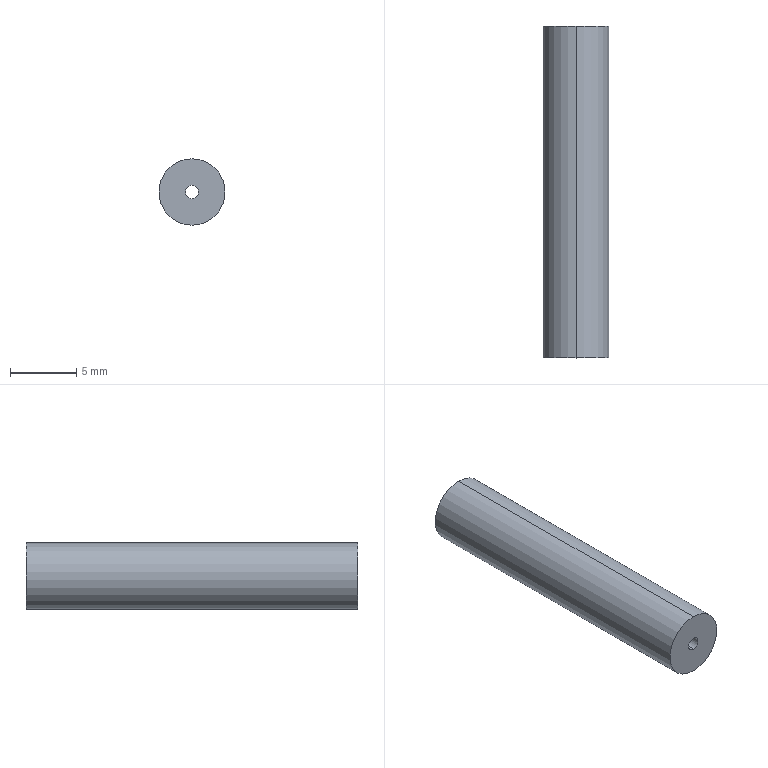Part | SolidWorks | features Extrusion 1, ICE 1 | 1 solid | 9 faces | box 5 x 25 x 5 mm | volume 326.726 mm3 | cylinder 6 | plane 3 | commonest cylinder face diameters 1 x2 3 x2 5 x2
STEP:
#1=CARTESIAN_POINT('',(0.,2.,0.5));
#2=VERTEX_POINT('',#1);
#3=CARTESIAN_POINT('',(0.,2.,-0.5));
#4=VERTEX_POINT('',#3);
#5=CARTESIAN_POINT('',(0.,2.,0.));
#6=DIRECTION('',(0.,-1.,0.));
#7=DIRECTION('',(0.,0.,-1.));
#8=AXIS2_PLACEMENT_3D('',#5,#6,#7);
#9=CIRCLE('',#8,0.5);
#10=EDGE_CURVE('',#2,#4,#9,.T.);
#11=ORIENTED_EDGE('',*,*,#10,.F.);
#12=CARTESIAN_POINT('',(0.,0.,0.5));
#13=VERTEX_POINT('',#12);
#14=CARTESIAN_POINT('',(0.,2.,0.5));
#15=DIRECTION('',(0.,-1.,0.));
#16=VECTOR('',#15,1000.);
#17=LINE('',#14,#16);
#18=EDGE_CURVE('',#2,#13,#17,.T.);
#19=ORIENTED_EDGE('',*,*,#18,.T.);
#20=CARTESIAN_POINT('',(0.,0.,-0.5));
#21=VERTEX_POINT('',#20);
#22=CARTESIAN_POINT('',(0.,0.,0.));
#23=DIRECTION('',(0.,-1.,0.));
#24=DIRECTION('',(0.,0.,-1.));
#25=AXIS2_PLACEMENT_3D('',#22,#23,#24);
#26=CIRCLE('',#25,0.5);
#27=EDGE_CURVE('',#13,#21,#26,.T.);
#28=ORIENTED_EDGE('',*,*,#27,.T.);
#29=CARTESIAN_POINT('',(0.,2.,-0.5));
#30=DIRECTION('',(0.,-1.,0.));
#31=VECTOR('',#30,1000.);
#32=LINE('',#29,#31);
#33=EDGE_CURVE('',#4,#21,#32,.T.);
#34=ORIENTED_EDGE('',*,*,#33,.F.);
#35=EDGE_LOOP('',(#11,#19,#28,#34));
#36=FACE_OUTER_BOUND('',#35,.T.);
#37=CARTESIAN_POINT('',(0.,2.,0.));
#38=DIRECTION('',(0.,-1.,0.));
#39=DIRECTION('',(0.,0.,-1.));
#40=AXIS2_PLACEMENT_3D('',#37,#38,#39);
#41=CYLINDRICAL_SURFACE('',#40,0.5);
#42=ADVANCED_FACE('',(#36),#41,.F.);
#43=CARTESIAN_POINT('',(0.,25.,2.5));
#44=VERTEX_POINT('',#43);
#45=CARTESIAN_POINT('',(0.,25.,-2.5));
#46=VERTEX_POINT('',#45);
#47=CARTESIAN_POINT('',(0.,25.,0.));
#48=DIRECTION('',(0.,1.,0.));
#49=DIRECTION('',(0.,0.,1.));
#50=AXIS2_PLACEMENT_3D('',#47,#48,#49);
#51=CIRCLE('',#50,2.5);
#52=EDGE_CURVE('',#44,#46,#51,.T.);
#53=ORIENTED_EDGE('',*,*,#52,.F.);
#54=CARTESIAN_POINT('',(0.,0.,2.5));
#55=VERTEX_POINT('',#54);
#56=CARTESIAN_POINT('',(0.,25.,2.5));
#57=DIRECTION('',(0.,-1.,0.));
#58=VECTOR('',#57,1000.);
#59=LINE('',#56,#58);
#60=EDGE_CURVE('',#44,#55,#59,.T.);
#61=ORIENTED_EDGE('',*,*,#60,.T.);
#62=CARTESIAN_POINT('',(0.,0.,-2.5));
#63=VERTEX_POINT('',#62);
#64=CARTESIAN_POINT('',(0.,0.,0.));
#65=DIRECTION('',(0.,1.,0.));
#66=DIRECTION('',(0.,0.,1.));
#67=AXIS2_PLACEMENT_3D('',#64,#65,#66);
#68=CIRCLE('',#67,2.5);
#69=EDGE_CURVE('',#55,#63,#68,.T.);
#70=ORIENTED_EDGE('',*,*,#69,.T.);
#71=CARTESIAN_POINT('',(0.,25.,-2.5));
#72=DIRECTION('',(0.,-1.,0.));
#73=VECTOR('',#72,1000.);
#74=LINE('',#71,#73);
#75=EDGE_CURVE('',#46,#63,#74,.T.);
#76=ORIENTED_EDGE('',*,*,#75,.F.);
#77=EDGE_LOOP('',(#53,#61,#70,#76));
#78=FACE_OUTER_BOUND('',#77,.T.);
#79=CARTESIAN_POINT('',(0.,25.,0.));
#80=DIRECTION('',(0.,-1.,0.));
#81=DIRECTION('',(0.,0.,-1.));
#82=AXIS2_PLACEMENT_3D('',#79,#80,#81);
#83=CYLINDRICAL_SURFACE('',#82,2.5);
#84=ADVANCED_FACE('',(#78),#83,.T.);
#85=CARTESIAN_POINT('',(0.,25.,-1.5));
#86=VERTEX_POINT('',#85);
#87=CARTESIAN_POINT('',(0.,25.,1.5));
#88=VERTEX_POINT('',#87);
#89=CARTESIAN_POINT('',(0.,25.,0.));
#90=DIRECTION('',(0.,1.,0.));
#91=DIRECTION('',(0.,0.,1.));
#92=AXIS2_PLACEMENT_3D('',#89,#90,#91);
#93=CIRCLE('',#92,1.5);
#94=EDGE_CURVE('',#86,#88,#93,.T.);
#95=ORIENTED_EDGE('',*,*,#94,.T.);
#96=CARTESIAN_POINT('',(0.,2.,1.5));
#97=VERTEX_POINT('',#96);
#98=CARTESIAN_POINT('',(0.,25.,1.5));
#99=DIRECTION('',(0.,-1.,0.));
#100=VECTOR('',#99,1000.);
#101=LINE('',#98,#100);
#102=EDGE_CURVE('',#88,#97,#101,.T.);
#103=ORIENTED_EDGE('',*,*,#102,.T.);
#104=CARTESIAN_POINT('',(0.,2.,-1.5));
#105=VERTEX_POINT('',#104);
#106=CARTESIAN_POINT('',(0.,2.,0.));
#107=DIRECTION('',(0.,-1.,0.));
#108=DIRECTION('',(0.,0.,-1.));
#109=AXIS2_PLACEMENT_3D('',#106,#107,#108);
#110=CIRCLE('',#109,1.5);
#111=EDGE_CURVE('',#97,#105,#110,.T.);
#112=ORIENTED_EDGE('',*,*,#111,.T.);
#113=CARTESIAN_POINT('',(0.,25.,-1.5));
#114=DIRECTION('',(0.,-1.,0.));
#115=VECTOR('',#114,1000.);
#116=LINE('',#113,#115);
#117=EDGE_CURVE('',#86,#105,#116,.T.);
#118=ORIENTED_EDGE('',*,*,#117,.F.);
#119=EDGE_LOOP('',(#95,#103,#112,#118));
#120=FACE_OUTER_BOUND('',#119,.T.);
#121=CARTESIAN_POINT('',(0.,25.,0.));
#122=DIRECTION('',(0.,-1.,0.));
#123=DIRECTION('',(0.,0.,-1.));
#124=AXIS2_PLACEMENT_3D('',#121,#122,#123);
#125=CYLINDRICAL_SURFACE('',#124,1.5);
#126=ADVANCED_FACE('',(#120),#125,.F.);
#127=ORIENTED_EDGE('',*,*,#102,.F.);
#128=CARTESIAN_POINT('',(0.,25.,0.));
#129=DIRECTION('',(0.,1.,0.));
#130=DIRECTION('',(0.,0.,1.));
#131=AXIS2_PLACEMENT_3D('',#128,#129,#130);
#132=CIRCLE('',#131,1.5);
#133=EDGE_CURVE('',#88,#86,#132,.T.);
#134=ORIENTED_EDGE('',*,*,#133,.T.);
#135=ORIENTED_EDGE('',*,*,#117,.T.);
#136=CARTESIAN_POINT('',(0.,2.,0.));
#137=DIRECTION('',(0.,-1.,0.));
#138=DIRECTION('',(0.,0.,-1.));
#139=AXIS2_PLACEMENT_3D('',#136,#137,#138);
#140=CIRCLE('',#139,1.5);
#141=EDGE_CURVE('',#105,#97,#140,.T.);
#142=ORIENTED_EDGE('',*,*,#141,.T.);
#143=EDGE_LOOP('',(#127,#134,#135,#142));
#144=FACE_OUTER_BOUND('',#143,.T.);
#145=CARTESIAN_POINT('',(0.,25.,0.));
#146=DIRECTION('',(0.,-1.,0.));
#147=DIRECTION('',(0.,0.,-1.));
#148=AXIS2_PLACEMENT_3D('',#145,#146,#147);
#149=CYLINDRICAL_SURFACE('',#148,1.5);
#150=ADVANCED_FACE('',(#144),#149,.F.);
#151=CARTESIAN_POINT('',(0.,25.,0.));
#152=DIRECTION('',(0.,1.,0.));
#153=DIRECTION('',(0.,0.,1.));
#154=AXIS2_PLACEMENT_3D('',#151,#152,#153);
#155=CIRCLE('',#154,2.5);
#156=EDGE_CURVE('',#46,#44,#155,.T.);
#157=ORIENTED_EDGE('',*,*,#156,.T.);
#158=ORIENTED_EDGE('',*,*,#52,.T.);
#159=EDGE_LOOP('',(#157,#158));
#160=FACE_OUTER_BOUND('',#159,.T.);
#161=ORIENTED_EDGE('',*,*,#94,.F.);
#162=ORIENTED_EDGE('',*,*,#133,.F.);
#163=EDGE_LOOP('',(#161,#162));
#164=FACE_BOUND('',#163,.T.);
#165=CARTESIAN_POINT('',(0.,25.,0.));
#166=DIRECTION('',(0.,1.,0.));
#167=DIRECTION('',(0.,0.,1.));
#168=AXIS2_PLACEMENT_3D('',#165,#166,#167);
#169=PLANE('',#168);
#170=ADVANCED_FACE('',(#160,#164),#169,.T.);
#171=CARTESIAN_POINT('',(0.,0.,0.));
#172=DIRECTION('',(0.,1.,0.));
#173=DIRECTION('',(0.,0.,1.));
#174=AXIS2_PLACEMENT_3D('',#171,#172,#173);
#175=CIRCLE('',#174,2.5);
#176=EDGE_CURVE('',#63,#55,#175,.T.);
#177=ORIENTED_EDGE('',*,*,#176,.F.);
#178=ORIENTED_EDGE('',*,*,#69,.F.);
#179=EDGE_LOOP('',(#177,#178));
#180=FACE_OUTER_BOUND('',#179,.T.);
#181=CARTESIAN_POINT('',(0.,0.,0.));
#182=DIRECTION('',(0.,-1.,0.));
#183=DIRECTION('',(0.,0.,-1.));
#184=AXIS2_PLACEMENT_3D('',#181,#182,#183);
#185=CIRCLE('',#184,0.5);
#186=EDGE_CURVE('',#21,#13,#185,.T.);
#187=ORIENTED_EDGE('',*,*,#186,.F.);
#188=ORIENTED_EDGE('',*,*,#27,.F.);
#189=EDGE_LOOP('',(#187,#188));
#190=FACE_BOUND('',#189,.T.);
#191=CARTESIAN_POINT('',(0.,0.,0.));
#192=DIRECTION('',(0.,1.,0.));
#193=DIRECTION('',(0.,0.,1.));
#194=AXIS2_PLACEMENT_3D('',#191,#192,#193);
#195=PLANE('',#194);
#196=ADVANCED_FACE('',(#180,#190),#195,.F.);
#197=ORIENTED_EDGE('',*,*,#60,.F.);
#198=ORIENTED_EDGE('',*,*,#156,.F.);
#199=ORIENTED_EDGE('',*,*,#75,.T.);
#200=ORIENTED_EDGE('',*,*,#176,.T.);
#201=EDGE_LOOP('',(#197,#198,#199,#200));
#202=FACE_OUTER_BOUND('',#201,.T.);
#203=CARTESIAN_POINT('',(0.,25.,0.));
#204=DIRECTION('',(0.,-1.,0.));
#205=DIRECTION('',(0.,0.,-1.));
#206=AXIS2_PLACEMENT_3D('',#203,#204,#205);
#207=CYLINDRICAL_SURFACE('',#206,2.5);
#208=ADVANCED_FACE('',(#202),#207,.T.);
#209=CARTESIAN_POINT('',(0.,2.,0.));
#210=DIRECTION('',(0.,-1.,0.));
#211=DIRECTION('',(0.,0.,-1.));
#212=AXIS2_PLACEMENT_3D('',#209,#210,#211);
#213=CIRCLE('',#212,0.5);
#214=EDGE_CURVE('',#4,#2,#213,.T.);
#215=ORIENTED_EDGE('',*,*,#214,.T.);
#216=ORIENTED_EDGE('',*,*,#10,.T.);
#217=EDGE_LOOP('',(#215,#216));
#218=FACE_BOUND('',#217,.T.);
#219=ORIENTED_EDGE('',*,*,#141,.F.);
#220=ORIENTED_EDGE('',*,*,#111,.F.);
#221=EDGE_LOOP('',(#219,#220));
#222=FACE_OUTER_BOUND('',#221,.T.);
#223=CARTESIAN_POINT('',(0.,2.,0.));
#224=DIRECTION('',(0.,-1.,0.));
#225=DIRECTION('',(0.,0.,-1.));
#226=AXIS2_PLACEMENT_3D('',#223,#224,#225);
#227=PLANE('',#226);
#228=ADVANCED_FACE('',(#218,#222),#227,.F.);
#229=ORIENTED_EDGE('',*,*,#18,.F.);
#230=ORIENTED_EDGE('',*,*,#214,.F.);
#231=ORIENTED_EDGE('',*,*,#33,.T.);
#232=ORIENTED_EDGE('',*,*,#186,.T.);
#233=EDGE_LOOP('',(#229,#230,#231,#232));
#234=FACE_OUTER_BOUND('',#233,.T.);
#235=CARTESIAN_POINT('',(0.,2.,0.));
#236=DIRECTION('',(0.,-1.,0.));
#237=DIRECTION('',(0.,0.,-1.));
#238=AXIS2_PLACEMENT_3D('',#235,#236,#237);
#239=CYLINDRICAL_SURFACE('',#238,0.5);
#240=ADVANCED_FACE('',(#234),#239,.F.);
#241=CLOSED_SHELL('',(#42,#84,#126,#150,#170,#196,#208,#228,#240));
#242=MANIFOLD_SOLID_BREP('',#241);
#243=CARTESIAN_POINT('',(0.,0.,0.));
#244=DIRECTION('',(0.,0.,1.));
#245=DIRECTION('',(1.,0.,0.));
#246=AXIS2_PLACEMENT_3D('',#243,#244,#245);
#247=(LENGTH_UNIT()NAMED_UNIT(*)SI_UNIT(.MILLI.,.METRE.));
#248=UNCERTAINTY_MEASURE_WITH_UNIT(LENGTH_MEASURE(0.00001),#247,'','');
#249=(NAMED_UNIT(*)PLANE_ANGLE_UNIT()SI_UNIT($,.RADIAN.));
#250=(NAMED_UNIT(*)SI_UNIT($,.STERADIAN.)SOLID_ANGLE_UNIT());
#251=(GEOMETRIC_REPRESENTATION_CONTEXT(3)GLOBAL_UNCERTAINTY_ASSIGNED_CONTEXT((#248))GLOBAL_UNIT_ASSIGNED_CONTEXT((#247,#249,#250))REPRESENTATION_CONTEXT('',''));
#252=ADVANCED_BREP_SHAPE_REPRESENTATION('',(#242,#246),#251);